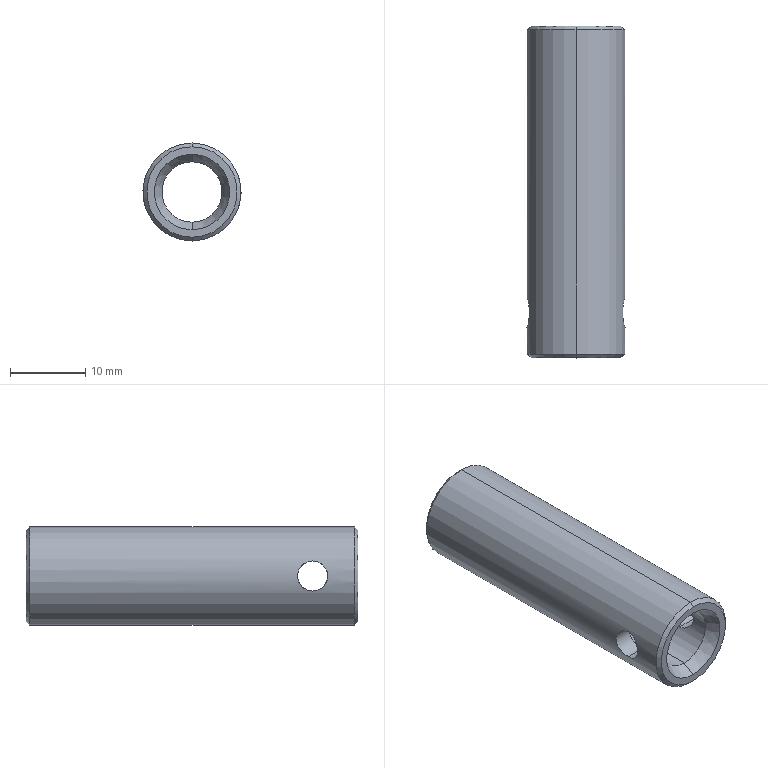Part | SolidWorks | features Chamfer 2, 3DProfileFeature 1, Extrusion 1, HoleWzd 1 | 1 solid | 18 faces | box 13 x 44 x 13 mm | volume 3507 mm3 | cone 8 | cylinder 8 | plane 2 | commonest cylinder face diameters 4 x4 8 x2 13 x2
STEP:
#1=CARTESIAN_POINT('',(0.,42.268,-4.));
#2=VERTEX_POINT('',#1);
#3=CARTESIAN_POINT('',(0.,42.268,4.));
#4=VERTEX_POINT('',#3);
#5=CARTESIAN_POINT('',(0.,42.268,0.));
#6=DIRECTION('',(0.,1.,0.));
#7=DIRECTION('',(0.,0.,1.));
#8=AXIS2_PLACEMENT_3D('',#5,#6,#7);
#9=CIRCLE('',#8,4.);
#10=EDGE_CURVE('',#2,#4,#9,.T.);
#11=ORIENTED_EDGE('',*,*,#10,.F.);
#12=CARTESIAN_POINT('',(0.,44.,-5.));
#13=VERTEX_POINT('',#12);
#14=CARTESIAN_POINT('',(0.,42.268,-4.));
#15=DIRECTION('',(0.,0.866,-0.5));
#16=VECTOR('',#15,1000.);
#17=LINE('',#14,#16);
#18=EDGE_CURVE('',#2,#13,#17,.T.);
#19=ORIENTED_EDGE('',*,*,#18,.T.);
#20=CARTESIAN_POINT('',(0.,44.,5.));
#21=VERTEX_POINT('',#20);
#22=CARTESIAN_POINT('',(0.,44.,0.));
#23=DIRECTION('',(0.,-1.,0.));
#24=DIRECTION('',(0.,0.,1.));
#25=AXIS2_PLACEMENT_3D('',#22,#23,#24);
#26=CIRCLE('',#25,5.);
#27=EDGE_CURVE('',#21,#13,#26,.T.);
#28=ORIENTED_EDGE('',*,*,#27,.F.);
#29=CARTESIAN_POINT('',(0.,42.268,4.));
#30=DIRECTION('',(0.,0.866,0.5));
#31=VECTOR('',#30,1000.);
#32=LINE('',#29,#31);
#33=EDGE_CURVE('',#4,#21,#32,.T.);
#34=ORIENTED_EDGE('',*,*,#33,.F.);
#35=EDGE_LOOP('',(#11,#19,#28,#34));
#36=FACE_OUTER_BOUND('',#35,.T.);
#37=CARTESIAN_POINT('',(0.,42.268,0.));
#38=DIRECTION('',(0.,1.,0.));
#39=DIRECTION('',(0.,0.,1.));
#40=AXIS2_PLACEMENT_3D('',#37,#38,#39);
#41=CONICAL_SURFACE('',#40,4.,0.5236);
#42=ADVANCED_FACE('',(#36),#41,.F.);
#43=CARTESIAN_POINT('',(0.,1.732,4.));
#44=VERTEX_POINT('',#43);
#45=CARTESIAN_POINT('',(0.,1.732,-4.));
#46=VERTEX_POINT('',#45);
#47=CARTESIAN_POINT('',(0.,1.732,0.));
#48=DIRECTION('',(0.,-1.,0.));
#49=DIRECTION('',(0.,0.,1.));
#50=AXIS2_PLACEMENT_3D('',#47,#48,#49);
#51=CIRCLE('',#50,4.);
#52=EDGE_CURVE('',#44,#46,#51,.T.);
#53=ORIENTED_EDGE('',*,*,#52,.F.);
#54=CARTESIAN_POINT('',(0.,0.,5.));
#55=VERTEX_POINT('',#54);
#56=CARTESIAN_POINT('',(0.,0.,5.));
#57=DIRECTION('',(0.,-0.866,0.5));
#58=VECTOR('',#57,1000.);
#59=LINE('',#56,#58);
#60=EDGE_CURVE('',#44,#55,#59,.T.);
#61=ORIENTED_EDGE('',*,*,#60,.T.);
#62=CARTESIAN_POINT('',(0.,0.,-5.));
#63=VERTEX_POINT('',#62);
#64=CARTESIAN_POINT('',(0.,0.,0.));
#65=DIRECTION('',(0.,1.,0.));
#66=DIRECTION('',(0.,0.,1.));
#67=AXIS2_PLACEMENT_3D('',#64,#65,#66);
#68=CIRCLE('',#67,5.);
#69=EDGE_CURVE('',#63,#55,#68,.T.);
#70=ORIENTED_EDGE('',*,*,#69,.F.);
#71=CARTESIAN_POINT('',(0.,0.,-5.));
#72=DIRECTION('',(0.,-0.866,-0.5));
#73=VECTOR('',#72,1000.);
#74=LINE('',#71,#73);
#75=EDGE_CURVE('',#46,#63,#74,.T.);
#76=ORIENTED_EDGE('',*,*,#75,.F.);
#77=EDGE_LOOP('',(#53,#61,#70,#76));
#78=FACE_OUTER_BOUND('',#77,.T.);
#79=CARTESIAN_POINT('',(0.,0.,0.));
#80=DIRECTION('',(0.,-1.,0.));
#81=DIRECTION('',(0.,0.,-1.));
#82=AXIS2_PLACEMENT_3D('',#79,#80,#81);
#83=CONICAL_SURFACE('',#82,5.,0.5236);
#84=ADVANCED_FACE('',(#78),#83,.F.);
#85=CARTESIAN_POINT('',(0.,44.,6.));
#86=VERTEX_POINT('',#85);
#87=CARTESIAN_POINT('',(0.,44.,-6.));
#88=VERTEX_POINT('',#87);
#89=CARTESIAN_POINT('',(0.,44.,0.));
#90=DIRECTION('',(0.,1.,0.));
#91=DIRECTION('',(0.,0.,1.));
#92=AXIS2_PLACEMENT_3D('',#89,#90,#91);
#93=CIRCLE('',#92,6.);
#94=EDGE_CURVE('',#86,#88,#93,.T.);
#95=ORIENTED_EDGE('',*,*,#94,.F.);
#96=CARTESIAN_POINT('',(0.,43.5,6.5));
#97=VERTEX_POINT('',#96);
#98=CARTESIAN_POINT('',(0.,44.,6.));
#99=DIRECTION('',(0.,-0.7071,0.7071));
#100=VECTOR('',#99,1000.);
#101=LINE('',#98,#100);
#102=EDGE_CURVE('',#86,#97,#101,.T.);
#103=ORIENTED_EDGE('',*,*,#102,.T.);
#104=CARTESIAN_POINT('',(0.,43.5,-6.5));
#105=VERTEX_POINT('',#104);
#106=CARTESIAN_POINT('',(0.,43.5,0.));
#107=DIRECTION('',(0.,-1.,0.));
#108=DIRECTION('',(0.,0.,1.));
#109=AXIS2_PLACEMENT_3D('',#106,#107,#108);
#110=CIRCLE('',#109,6.5);
#111=EDGE_CURVE('',#105,#97,#110,.T.);
#112=ORIENTED_EDGE('',*,*,#111,.F.);
#113=CARTESIAN_POINT('',(0.,44.,-6.));
#114=DIRECTION('',(0.,-0.7071,-0.7071));
#115=VECTOR('',#114,1000.);
#116=LINE('',#113,#115);
#117=EDGE_CURVE('',#88,#105,#116,.T.);
#118=ORIENTED_EDGE('',*,*,#117,.F.);
#119=EDGE_LOOP('',(#95,#103,#112,#118));
#120=FACE_OUTER_BOUND('',#119,.T.);
#121=CARTESIAN_POINT('',(0.,44.,0.));
#122=DIRECTION('',(0.,-1.,0.));
#123=DIRECTION('',(0.,0.,-1.));
#124=AXIS2_PLACEMENT_3D('',#121,#122,#123);
#125=CONICAL_SURFACE('',#124,6.,0.7854);
#126=ADVANCED_FACE('',(#120),#125,.T.);
#127=CARTESIAN_POINT('',(0.,0.,-6.));
#128=VERTEX_POINT('',#127);
#129=CARTESIAN_POINT('',(0.,0.,6.));
#130=VERTEX_POINT('',#129);
#131=CARTESIAN_POINT('',(0.,0.,0.));
#132=DIRECTION('',(0.,-1.,0.));
#133=DIRECTION('',(0.,0.,1.));
#134=AXIS2_PLACEMENT_3D('',#131,#132,#133);
#135=CIRCLE('',#134,6.);
#136=EDGE_CURVE('',#128,#130,#135,.T.);
#137=ORIENTED_EDGE('',*,*,#136,.F.);
#138=CARTESIAN_POINT('',(0.,0.5,-6.5));
#139=VERTEX_POINT('',#138);
#140=CARTESIAN_POINT('',(0.,0.5,-6.5));
#141=DIRECTION('',(0.,0.7071,-0.7071));
#142=VECTOR('',#141,1000.);
#143=LINE('',#140,#142);
#144=EDGE_CURVE('',#128,#139,#143,.T.);
#145=ORIENTED_EDGE('',*,*,#144,.T.);
#146=CARTESIAN_POINT('',(0.,0.5,6.5));
#147=VERTEX_POINT('',#146);
#148=CARTESIAN_POINT('',(0.,0.5,0.));
#149=DIRECTION('',(0.,1.,0.));
#150=DIRECTION('',(0.,0.,1.));
#151=AXIS2_PLACEMENT_3D('',#148,#149,#150);
#152=CIRCLE('',#151,6.5);
#153=EDGE_CURVE('',#147,#139,#152,.T.);
#154=ORIENTED_EDGE('',*,*,#153,.F.);
#155=CARTESIAN_POINT('',(0.,0.5,6.5));
#156=DIRECTION('',(0.,0.7071,0.7071));
#157=VECTOR('',#156,1000.);
#158=LINE('',#155,#157);
#159=EDGE_CURVE('',#130,#147,#158,.T.);
#160=ORIENTED_EDGE('',*,*,#159,.F.);
#161=EDGE_LOOP('',(#137,#145,#154,#160));
#162=FACE_OUTER_BOUND('',#161,.T.);
#163=CARTESIAN_POINT('',(0.,0.5,0.));
#164=DIRECTION('',(0.,1.,0.));
#165=DIRECTION('',(0.,0.,1.));
#166=AXIS2_PLACEMENT_3D('',#163,#164,#165);
#167=CONICAL_SURFACE('',#166,6.5,0.7854);
#168=ADVANCED_FACE('',(#162),#167,.T.);
#169=CARTESIAN_POINT('',(-6.185,6.,2.));
#170=VERTEX_POINT('',#169);
#171=CARTESIAN_POINT('',(-6.185,6.,-2.));
#172=VERTEX_POINT('',#171);
#173=CARTESIAN_POINT('',(-6.185,6.,2.));
#174=CARTESIAN_POINT('',(-6.185,5.868,2.));
#175=CARTESIAN_POINT('',(-6.189,5.738,1.987));
#176=CARTESIAN_POINT('',(-6.205,5.48,1.936));
#177=CARTESIAN_POINT('',(-6.217,5.352,1.897));
#178=CARTESIAN_POINT('',(-6.262,4.991,1.746));
#179=CARTESIAN_POINT('',(-6.303,4.769,1.598));
#180=CARTESIAN_POINT('',(-6.365,4.494,1.323));
#181=CARTESIAN_POINT('',(-6.385,4.41,1.221));
#182=CARTESIAN_POINT('',(-6.423,4.265,1.004));
#183=CARTESIAN_POINT('',(-6.44,4.204,0.8894));
#184=CARTESIAN_POINT('',(-6.469,4.103,0.6479));
#185=CARTESIAN_POINT('',(-6.48,4.064,0.5202));
#186=CARTESIAN_POINT('',(-6.496,4.013,0.2629));
#187=CARTESIAN_POINT('',(-6.5,4.,0.1321));
#188=CARTESIAN_POINT('',(-6.5,4.,-0.1339));
#189=CARTESIAN_POINT('',(-6.496,4.013,-0.2646));
#190=CARTESIAN_POINT('',(-6.48,4.065,-0.5213));
#191=CARTESIAN_POINT('',(-6.469,4.104,-0.6488));
#192=CARTESIAN_POINT('',(-6.44,4.204,-0.8906));
#193=CARTESIAN_POINT('',(-6.423,4.266,-1.005));
#194=CARTESIAN_POINT('',(-6.385,4.411,-1.222));
#195=CARTESIAN_POINT('',(-6.364,4.495,-1.324));
#196=CARTESIAN_POINT('',(-6.303,4.77,-1.599));
#197=CARTESIAN_POINT('',(-6.262,4.992,-1.747));
#198=CARTESIAN_POINT('',(-6.217,5.353,-1.897));
#199=CARTESIAN_POINT('',(-6.205,5.48,-1.936));
#200=CARTESIAN_POINT('',(-6.189,5.738,-1.987));
#201=CARTESIAN_POINT('',(-6.185,5.869,-2.));
#202=CARTESIAN_POINT('',(-6.185,6.,-2.));
#203=B_SPLINE_CURVE_WITH_KNOTS('',3,(#173,#174,#175,#176,#177,#178,#179,#180,#181,#182,#183,#184,#185,#186,#187,#188,#189,#190,#191,#192,#193,#194,#195,#196,#197,#198,#199,#200,#201,#202),.UNSPECIFIED.,.F.,.F.,(4,2,2,2,2,2,2,2,2,2,2,2,2,2,4),(0.009436,0.009829,0.01022,0.01101,0.0114,0.0118,0.01219,0.01258,0.01298,0.01337,0.01376,0.01415,0.01494,0.01533,0.01573),.UNSPECIFIED.);
#204=EDGE_CURVE('',#170,#172,#203,.T.);
#205=ORIENTED_EDGE('',*,*,#204,.F.);
#206=CARTESIAN_POINT('',(-3.464,6.,2.));
#207=VERTEX_POINT('',#206);
#208=CARTESIAN_POINT('',(6.5,6.,2.));
#209=DIRECTION('',(1.,0.,0.));
#210=VECTOR('',#209,1000.);
#211=LINE('',#208,#210);
#212=EDGE_CURVE('',#170,#207,#211,.T.);
#213=ORIENTED_EDGE('',*,*,#212,.T.);
#214=CARTESIAN_POINT('',(-3.464,6.,-2.));
#215=VERTEX_POINT('',#214);
#216=CARTESIAN_POINT('',(-3.464,6.,2.));
#217=CARTESIAN_POINT('',(-3.464,5.868,2.));
#218=CARTESIAN_POINT('',(-3.472,5.733,1.986));
#219=CARTESIAN_POINT('',(-3.501,5.474,1.934));
#220=CARTESIAN_POINT('',(-3.523,5.348,1.895));
#221=CARTESIAN_POINT('',(-3.576,5.105,1.794));
#222=CARTESIAN_POINT('',(-3.606,4.991,1.732));
#223=CARTESIAN_POINT('',(-3.672,4.778,1.588));
#224=CARTESIAN_POINT('',(-3.707,4.677,1.505));
#225=CARTESIAN_POINT('',(-3.776,4.495,1.324));
#226=CARTESIAN_POINT('',(-3.81,4.413,1.225));
#227=CARTESIAN_POINT('',(-3.872,4.269,1.01));
#228=CARTESIAN_POINT('',(-3.901,4.206,0.8936));
#229=CARTESIAN_POINT('',(-3.972,4.055,0.5337));
#230=CARTESIAN_POINT('',(-4.,4.,0.2665));
#231=CARTESIAN_POINT('',(-4.,4.,-0.1307));
#232=CARTESIAN_POINT('',(-3.993,4.013,-0.265));
#233=CARTESIAN_POINT('',(-3.967,4.066,-0.5254));
#234=CARTESIAN_POINT('',(-3.949,4.104,-0.651));
#235=CARTESIAN_POINT('',(-3.877,4.257,-1.015));
#236=CARTESIAN_POINT('',(-3.81,4.404,-1.233));
#237=CARTESIAN_POINT('',(-3.707,4.678,-1.507));
#238=CARTESIAN_POINT('',(-3.672,4.777,-1.588));
#239=CARTESIAN_POINT('',(-3.607,4.991,-1.732));
#240=CARTESIAN_POINT('',(-3.575,5.107,-1.794));
#241=CARTESIAN_POINT('',(-3.523,5.347,-1.895));
#242=CARTESIAN_POINT('',(-3.502,5.471,-1.933));
#243=CARTESIAN_POINT('',(-3.472,5.731,-1.986));
#244=CARTESIAN_POINT('',(-3.464,5.866,-2.));
#245=CARTESIAN_POINT('',(-3.464,6.,-2.));
#246=B_SPLINE_CURVE_WITH_KNOTS('',3,(#216,#217,#218,#219,#220,#221,#222,#223,#224,#225,#226,#227,#228,#229,#230,#231,#232,#233,#234,#235,#236,#237,#238,#239,#240,#241,#242,#243,#244,#245),.UNSPECIFIED.,.F.,.F.,(4,2,2,2,2,2,2,2,2,2,2,2,2,2,4),(0.006361,0.006758,0.007155,0.007552,0.007949,0.008346,0.008742,0.009536,0.009933,0.01033,0.01112,0.01152,0.01192,0.01231,0.01271),.UNSPECIFIED.);
#247=EDGE_CURVE('',#207,#215,#246,.T.);
#248=ORIENTED_EDGE('',*,*,#247,.T.);
#249=CARTESIAN_POINT('',(6.5,6.,-2.));
#250=DIRECTION('',(1.,0.,0.));
#251=VECTOR('',#250,1000.);
#252=LINE('',#249,#251);
#253=EDGE_CURVE('',#172,#215,#252,.T.);
#254=ORIENTED_EDGE('',*,*,#253,.F.);
#255=EDGE_LOOP('',(#205,#213,#248,#254));
#256=FACE_OUTER_BOUND('',#255,.T.);
#257=CARTESIAN_POINT('',(6.5,6.,0.));
#258=DIRECTION('',(1.,0.,0.));
#259=DIRECTION('',(0.,0.,-1.));
#260=AXIS2_PLACEMENT_3D('',#257,#258,#259);
#261=CYLINDRICAL_SURFACE('',#260,2.);
#262=ADVANCED_FACE('',(#256),#261,.F.);
#263=CARTESIAN_POINT('',(3.464,6.,-2.));
#264=VERTEX_POINT('',#263);
#265=CARTESIAN_POINT('',(3.464,6.,2.));
#266=VERTEX_POINT('',#265);
#267=CARTESIAN_POINT('',(3.464,6.,-2.));
#268=CARTESIAN_POINT('',(3.464,5.865,-2.));
#269=CARTESIAN_POINT('',(3.472,5.733,-1.987));
#270=CARTESIAN_POINT('',(3.501,5.475,-1.934));
#271=CARTESIAN_POINT('',(3.523,5.347,-1.895));
#272=CARTESIAN_POINT('',(3.602,4.986,-1.743));
#273=CARTESIAN_POINT('',(3.673,4.768,-1.596));
#274=CARTESIAN_POINT('',(3.81,4.405,-1.233));
#275=CARTESIAN_POINT('',(3.877,4.257,-1.014));
#276=CARTESIAN_POINT('',(3.948,4.105,-0.6539));
#277=CARTESIAN_POINT('',(3.967,4.066,-0.5256));
#278=CARTESIAN_POINT('',(3.993,4.013,-0.2661));
#279=CARTESIAN_POINT('',(4.,4.,-0.1346));
#280=CARTESIAN_POINT('',(4.,4.,0.132));
#281=CARTESIAN_POINT('',(3.993,4.013,0.2666));
#282=CARTESIAN_POINT('',(3.967,4.066,0.5257));
#283=CARTESIAN_POINT('',(3.948,4.105,0.653));
#284=CARTESIAN_POINT('',(3.9,4.207,0.8959));
#285=CARTESIAN_POINT('',(3.872,4.269,1.01));
#286=CARTESIAN_POINT('',(3.809,4.414,1.225));
#287=CARTESIAN_POINT('',(3.775,4.497,1.326));
#288=CARTESIAN_POINT('',(3.672,4.77,1.598));
#289=CARTESIAN_POINT('',(3.601,4.989,1.745));
#290=CARTESIAN_POINT('',(3.523,5.348,1.895));
#291=CARTESIAN_POINT('',(3.501,5.475,1.934));
#292=CARTESIAN_POINT('',(3.472,5.736,1.987));
#293=CARTESIAN_POINT('',(3.464,5.867,2.));
#294=CARTESIAN_POINT('',(3.464,6.,2.));
#295=B_SPLINE_CURVE_WITH_KNOTS('',3,(#267,#268,#269,#270,#271,#272,#273,#274,#275,#276,#277,#278,#279,#280,#281,#282,#283,#284,#285,#286,#287,#288,#289,#290,#291,#292,#293,#294),.UNSPECIFIED.,.F.,.F.,(4,2,2,2,2,2,2,2,2,2,2,2,2,4),(0.,0.0003976,0.0007951,0.00159,0.002385,0.002783,0.003181,0.003578,0.003976,0.004373,0.004771,0.005566,0.005964,0.006361),.UNSPECIFIED.);
#296=EDGE_CURVE('',#264,#266,#295,.T.);
#297=ORIENTED_EDGE('',*,*,#296,.T.);
#298=CARTESIAN_POINT('',(6.185,6.,2.));
#299=VERTEX_POINT('',#298);
#300=CARTESIAN_POINT('',(6.5,6.,2.));
#301=DIRECTION('',(1.,0.,0.));
#302=VECTOR('',#301,1000.);
#303=LINE('',#300,#302);
#304=EDGE_CURVE('',#266,#299,#303,.T.);
#305=ORIENTED_EDGE('',*,*,#304,.T.);
#306=CARTESIAN_POINT('',(6.185,6.,-2.));
#307=VERTEX_POINT('',#306);
#308=CARTESIAN_POINT('',(6.185,6.,-2.));
#309=CARTESIAN_POINT('',(6.185,5.867,-2.));
#310=CARTESIAN_POINT('',(6.189,5.736,-1.987));
#311=CARTESIAN_POINT('',(6.205,5.48,-1.936));
#312=CARTESIAN_POINT('',(6.217,5.352,-1.897));
#313=CARTESIAN_POINT('',(6.247,5.11,-1.796));
#314=CARTESIAN_POINT('',(6.265,4.996,-1.735));
#315=CARTESIAN_POINT('',(6.303,4.779,-1.589));
#316=CARTESIAN_POINT('',(6.324,4.677,-1.506));
#317=CARTESIAN_POINT('',(6.385,4.402,-1.231));
#318=CARTESIAN_POINT('',(6.426,4.254,-1.009));
#319=CARTESIAN_POINT('',(6.469,4.103,-0.6481));
#320=CARTESIAN_POINT('',(6.48,4.065,-0.5212));
#321=CARTESIAN_POINT('',(6.496,4.013,-0.2626));
#322=CARTESIAN_POINT('',(6.5,4.,-0.1323));
#323=CARTESIAN_POINT('',(6.5,4.,0.1305));
#324=CARTESIAN_POINT('',(6.496,4.013,0.2639));
#325=CARTESIAN_POINT('',(6.48,4.065,0.5212));
#326=CARTESIAN_POINT('',(6.469,4.103,0.6463));
#327=CARTESIAN_POINT('',(6.426,4.254,1.011));
#328=CARTESIAN_POINT('',(6.385,4.402,1.231));
#329=CARTESIAN_POINT('',(6.324,4.679,1.507));
#330=CARTESIAN_POINT('',(6.303,4.779,1.589));
#331=CARTESIAN_POINT('',(6.265,4.995,1.734));
#332=CARTESIAN_POINT('',(6.247,5.112,1.797));
#333=CARTESIAN_POINT('',(6.217,5.353,1.897));
#334=CARTESIAN_POINT('',(6.205,5.478,1.935));
#335=CARTESIAN_POINT('',(6.189,5.736,1.987));
#336=CARTESIAN_POINT('',(6.185,5.869,2.));
#337=CARTESIAN_POINT('',(6.185,6.,2.));
#338=B_SPLINE_CURVE_WITH_KNOTS('',3,(#308,#309,#310,#311,#312,#313,#314,#315,#316,#317,#318,#319,#320,#321,#322,#323,#324,#325,#326,#327,#328,#329,#330,#331,#332,#333,#334,#335,#336,#337),.UNSPECIFIED.,.F.,.F.,(4,2,2,2,2,2,2,2,2,2,2,2,2,2,4),(0.,0.0003932,0.0007864,0.00118,0.001573,0.002359,0.002752,0.003146,0.003539,0.003932,0.004718,0.005112,0.005505,0.005898,0.006291),.UNSPECIFIED.);
#339=EDGE_CURVE('',#307,#299,#338,.T.);
#340=ORIENTED_EDGE('',*,*,#339,.F.);
#341=CARTESIAN_POINT('',(6.5,6.,-2.));
#342=DIRECTION('',(1.,0.,0.));
#343=VECTOR('',#342,1000.);
#344=LINE('',#341,#343);
#345=EDGE_CURVE('',#264,#307,#344,.T.);
#346=ORIENTED_EDGE('',*,*,#345,.F.);
#347=EDGE_LOOP('',(#297,#305,#340,#346));
#348=FACE_OUTER_BOUND('',#347,.T.);
#349=CARTESIAN_POINT('',(6.5,6.,0.));
#350=DIRECTION('',(1.,0.,0.));
#351=DIRECTION('',(0.,0.,-1.));
#352=AXIS2_PLACEMENT_3D('',#349,#350,#351);
#353=CYLINDRICAL_SURFACE('',#352,2.);
#354=ADVANCED_FACE('',(#348),#353,.F.);
#355=CARTESIAN_POINT('',(-3.464,6.,-2.));
#356=CARTESIAN_POINT('',(-3.464,6.135,-2.));
#357=CARTESIAN_POINT('',(-3.472,6.267,-1.987));
#358=CARTESIAN_POINT('',(-3.501,6.525,-1.934));
#359=CARTESIAN_POINT('',(-3.523,6.653,-1.895));
#360=CARTESIAN_POINT('',(-3.602,7.014,-1.743));
#361=CARTESIAN_POINT('',(-3.673,7.232,-1.596));
#362=CARTESIAN_POINT('',(-3.81,7.595,-1.233));
#363=CARTESIAN_POINT('',(-3.877,7.743,-1.014));
#364=CARTESIAN_POINT('',(-3.948,7.895,-0.6539));
#365=CARTESIAN_POINT('',(-3.967,7.934,-0.5256));
#366=CARTESIAN_POINT('',(-3.993,7.987,-0.2661));
#367=CARTESIAN_POINT('',(-4.,8.,-0.1346));
#368=CARTESIAN_POINT('',(-4.,8.,0.132));
#369=CARTESIAN_POINT('',(-3.993,7.987,0.2666));
#370=CARTESIAN_POINT('',(-3.967,7.934,0.5257));
#371=CARTESIAN_POINT('',(-3.948,7.895,0.653));
#372=CARTESIAN_POINT('',(-3.9,7.793,0.8959));
#373=CARTESIAN_POINT('',(-3.872,7.731,1.01));
#374=CARTESIAN_POINT('',(-3.809,7.586,1.225));
#375=CARTESIAN_POINT('',(-3.775,7.503,1.326));
#376=CARTESIAN_POINT('',(-3.672,7.23,1.598));
#377=CARTESIAN_POINT('',(-3.601,7.011,1.745));
#378=CARTESIAN_POINT('',(-3.523,6.652,1.895));
#379=CARTESIAN_POINT('',(-3.501,6.525,1.934));
#380=CARTESIAN_POINT('',(-3.472,6.264,1.987));
#381=CARTESIAN_POINT('',(-3.464,6.133,2.));
#382=CARTESIAN_POINT('',(-3.464,6.,2.));
#383=B_SPLINE_CURVE_WITH_KNOTS('',3,(#355,#356,#357,#358,#359,#360,#361,#362,#363,#364,#365,#366,#367,#368,#369,#370,#371,#372,#373,#374,#375,#376,#377,#378,#379,#380,#381,#382),.UNSPECIFIED.,.F.,.F.,(4,2,2,2,2,2,2,2,2,2,2,2,2,4),(0.,0.0003976,0.0007951,0.00159,0.002385,0.002783,0.003181,0.003578,0.003976,0.004373,0.004771,0.005566,0.005964,0.006361),.UNSPECIFIED.);
#384=EDGE_CURVE('',#215,#207,#383,.T.);
#385=ORIENTED_EDGE('',*,*,#384,.F.);
#386=ORIENTED_EDGE('',*,*,#247,.F.);
#387=EDGE_LOOP('',(#385,#386));
#388=FACE_BOUND('',#387,.T.);
#389=ORIENTED_EDGE('',*,*,#10,.T.);
#390=CARTESIAN_POINT('',(0.,44.,4.));
#391=DIRECTION('',(0.,-1.,0.));
#392=VECTOR('',#391,1000.);
#393=LINE('',#390,#392);
#394=EDGE_CURVE('',#4,#44,#393,.T.);
#395=ORIENTED_EDGE('',*,*,#394,.T.);
#396=ORIENTED_EDGE('',*,*,#52,.T.);
#397=CARTESIAN_POINT('',(0.,44.,-4.));
#398=DIRECTION('',(0.,-1.,0.));
#399=VECTOR('',#398,1000.);
#400=LINE('',#397,#399);
#401=EDGE_CURVE('',#2,#46,#400,.T.);
#402=ORIENTED_EDGE('',*,*,#401,.F.);
#403=EDGE_LOOP('',(#389,#395,#396,#402));
#404=FACE_OUTER_BOUND('',#403,.T.);
#405=CARTESIAN_POINT('',(0.,44.,0.));
#406=DIRECTION('',(0.,-1.,0.));
#407=DIRECTION('',(0.,0.,-1.));
#408=AXIS2_PLACEMENT_3D('',#405,#406,#407);
#409=CYLINDRICAL_SURFACE('',#408,4.);
#410=ADVANCED_FACE('',(#388,#404),#409,.F.);
#411=ORIENTED_EDGE('',*,*,#339,.T.);
#412=CARTESIAN_POINT('',(6.185,6.,2.));
#413=CARTESIAN_POINT('',(6.185,6.262,2.));
#414=CARTESIAN_POINT('',(6.202,6.527,1.947));
#415=CARTESIAN_POINT('',(6.247,6.888,1.797));
#416=CARTESIAN_POINT('',(6.265,7.005,1.734));
#417=CARTESIAN_POINT('',(6.303,7.221,1.589));
#418=CARTESIAN_POINT('',(6.324,7.322,1.507));
#419=CARTESIAN_POINT('',(6.385,7.599,1.23));
#420=CARTESIAN_POINT('',(6.425,7.745,1.012));
#421=CARTESIAN_POINT('',(6.469,7.897,0.6464));
#422=CARTESIAN_POINT('',(6.48,7.935,0.5213));
#423=CARTESIAN_POINT('',(6.496,7.987,0.2649));
#424=CARTESIAN_POINT('',(6.5,8.,0.1318));
#425=CARTESIAN_POINT('',(6.5,8.,-0.1318));
#426=CARTESIAN_POINT('',(6.496,7.987,-0.2621));
#427=CARTESIAN_POINT('',(6.48,7.936,-0.52));
#428=CARTESIAN_POINT('',(6.469,7.897,-0.6476));
#429=CARTESIAN_POINT('',(6.426,7.746,-1.009));
#430=CARTESIAN_POINT('',(6.385,7.598,-1.231));
#431=CARTESIAN_POINT('',(6.324,7.323,-1.506));
#432=CARTESIAN_POINT('',(6.303,7.221,-1.59));
#433=CARTESIAN_POINT('',(6.265,7.004,-1.735));
#434=CARTESIAN_POINT('',(6.247,6.89,-1.796));
#435=CARTESIAN_POINT('',(6.217,6.649,-1.896));
#436=CARTESIAN_POINT('',(6.205,6.521,-1.935));
#437=CARTESIAN_POINT('',(6.189,6.264,-1.987));
#438=CARTESIAN_POINT('',(6.185,6.133,-2.));
#439=CARTESIAN_POINT('',(6.185,6.,-2.));
#440=B_SPLINE_CURVE_WITH_KNOTS('',3,(#412,#413,#414,#415,#416,#417,#418,#419,#420,#421,#422,#423,#424,#425,#426,#427,#428,#429,#430,#431,#432,#433,#434,#435,#436,#437,#438,#439),.UNSPECIFIED.,.F.,.F.,(4,2,2,2,2,2,2,2,2,2,2,2,2,4),(0.006291,0.007077,0.00747,0.007864,0.00865,0.009043,0.009436,0.009829,0.01022,0.01101,0.0114,0.01179,0.01219,0.01258),.UNSPECIFIED.);
#441=EDGE_CURVE('',#299,#307,#440,.T.);
#442=ORIENTED_EDGE('',*,*,#441,.T.);
#443=EDGE_LOOP('',(#411,#442));
#444=FACE_BOUND('',#443,.T.);
#445=ORIENTED_EDGE('',*,*,#111,.T.);
#446=CARTESIAN_POINT('',(0.,44.,6.5));
#447=DIRECTION('',(0.,-1.,0.));
#448=VECTOR('',#447,1000.);
#449=LINE('',#446,#448);
#450=EDGE_CURVE('',#97,#147,#449,.T.);
#451=ORIENTED_EDGE('',*,*,#450,.T.);
#452=ORIENTED_EDGE('',*,*,#153,.T.);
#453=CARTESIAN_POINT('',(0.,44.,-6.5));
#454=DIRECTION('',(0.,-1.,0.));
#455=VECTOR('',#454,1000.);
#456=LINE('',#453,#455);
#457=EDGE_CURVE('',#105,#139,#456,.T.);
#458=ORIENTED_EDGE('',*,*,#457,.F.);
#459=EDGE_LOOP('',(#445,#451,#452,#458));
#460=FACE_OUTER_BOUND('',#459,.T.);
#461=CARTESIAN_POINT('',(0.,44.,0.));
#462=DIRECTION('',(0.,-1.,0.));
#463=DIRECTION('',(0.,0.,-1.));
#464=AXIS2_PLACEMENT_3D('',#461,#462,#463);
#465=CYLINDRICAL_SURFACE('',#464,6.5);
#466=ADVANCED_FACE('',(#444,#460),#465,.T.);
#467=ORIENTED_EDGE('',*,*,#27,.T.);
#468=CARTESIAN_POINT('',(0.,44.,0.));
#469=DIRECTION('',(0.,-1.,0.));
#470=DIRECTION('',(0.,0.,1.));
#471=AXIS2_PLACEMENT_3D('',#468,#469,#470);
#472=CIRCLE('',#471,5.);
#473=EDGE_CURVE('',#13,#21,#472,.T.);
#474=ORIENTED_EDGE('',*,*,#473,.T.);
#475=EDGE_LOOP('',(#467,#474));
#476=FACE_BOUND('',#475,.T.);
#477=CARTESIAN_POINT('',(0.,44.,0.));
#478=DIRECTION('',(0.,1.,0.));
#479=DIRECTION('',(0.,0.,1.));
#480=AXIS2_PLACEMENT_3D('',#477,#478,#479);
#481=CIRCLE('',#480,6.);
#482=EDGE_CURVE('',#88,#86,#481,.T.);
#483=ORIENTED_EDGE('',*,*,#482,.T.);
#484=ORIENTED_EDGE('',*,*,#94,.T.);
#485=EDGE_LOOP('',(#483,#484));
#486=FACE_OUTER_BOUND('',#485,.T.);
#487=CARTESIAN_POINT('',(0.,44.,0.));
#488=DIRECTION('',(0.,1.,0.));
#489=DIRECTION('',(0.,0.,1.));
#490=AXIS2_PLACEMENT_3D('',#487,#488,#489);
#491=PLANE('',#490);
#492=ADVANCED_FACE('',(#476,#486),#491,.T.);
#493=ORIENTED_EDGE('',*,*,#69,.T.);
#494=CARTESIAN_POINT('',(0.,0.,0.));
#495=DIRECTION('',(0.,1.,0.));
#496=DIRECTION('',(0.,0.,1.));
#497=AXIS2_PLACEMENT_3D('',#494,#495,#496);
#498=CIRCLE('',#497,5.);
#499=EDGE_CURVE('',#55,#63,#498,.T.);
#500=ORIENTED_EDGE('',*,*,#499,.T.);
#501=EDGE_LOOP('',(#493,#500));
#502=FACE_BOUND('',#501,.T.);
#503=CARTESIAN_POINT('',(0.,0.,0.));
#504=DIRECTION('',(0.,-1.,0.));
#505=DIRECTION('',(0.,0.,1.));
#506=AXIS2_PLACEMENT_3D('',#503,#504,#505);
#507=CIRCLE('',#506,6.);
#508=EDGE_CURVE('',#130,#128,#507,.T.);
#509=ORIENTED_EDGE('',*,*,#508,.T.);
#510=ORIENTED_EDGE('',*,*,#136,.T.);
#511=EDGE_LOOP('',(#509,#510));
#512=FACE_OUTER_BOUND('',#511,.T.);
#513=CARTESIAN_POINT('',(0.,0.,0.));
#514=DIRECTION('',(0.,1.,0.));
#515=DIRECTION('',(0.,0.,1.));
#516=AXIS2_PLACEMENT_3D('',#513,#514,#515);
#517=PLANE('',#516);
#518=ADVANCED_FACE('',(#502,#512),#517,.F.);
#519=ORIENTED_EDGE('',*,*,#450,.F.);
#520=CARTESIAN_POINT('',(0.,43.5,0.));
#521=DIRECTION('',(0.,-1.,0.));
#522=DIRECTION('',(0.,0.,1.));
#523=AXIS2_PLACEMENT_3D('',#520,#521,#522);
#524=CIRCLE('',#523,6.5);
#525=EDGE_CURVE('',#97,#105,#524,.T.);
#526=ORIENTED_EDGE('',*,*,#525,.T.);
#527=ORIENTED_EDGE('',*,*,#457,.T.);
#528=CARTESIAN_POINT('',(0.,0.5,0.));
#529=DIRECTION('',(0.,1.,0.));
#530=DIRECTION('',(0.,0.,1.));
#531=AXIS2_PLACEMENT_3D('',#528,#529,#530);
#532=CIRCLE('',#531,6.5);
#533=EDGE_CURVE('',#139,#147,#532,.T.);
#534=ORIENTED_EDGE('',*,*,#533,.T.);
#535=EDGE_LOOP('',(#519,#526,#527,#534));
#536=FACE_OUTER_BOUND('',#535,.T.);
#537=CARTESIAN_POINT('',(-6.185,6.,-2.));
#538=CARTESIAN_POINT('',(-6.185,6.131,-2.));
#539=CARTESIAN_POINT('',(-6.189,6.265,-1.987));
#540=CARTESIAN_POINT('',(-6.205,6.522,-1.935));
#541=CARTESIAN_POINT('',(-6.217,6.647,-1.897));
#542=CARTESIAN_POINT('',(-6.262,7.011,-1.745));
#543=CARTESIAN_POINT('',(-6.303,7.231,-1.598));
#544=CARTESIAN_POINT('',(-6.365,7.507,-1.321));
#545=CARTESIAN_POINT('',(-6.385,7.589,-1.221));
#546=CARTESIAN_POINT('',(-6.423,7.734,-1.005));
#547=CARTESIAN_POINT('',(-6.44,7.797,-0.8878));
#548=CARTESIAN_POINT('',(-6.469,7.897,-0.6468));
#549=CARTESIAN_POINT('',(-6.48,7.935,-0.522));
#550=CARTESIAN_POINT('',(-6.496,7.987,-0.2636));
#551=CARTESIAN_POINT('',(-6.5,8.,-0.1309));
#552=CARTESIAN_POINT('',(-6.5,8.,0.2621));
#553=CARTESIAN_POINT('',(-6.483,7.947,0.5267));
#554=CARTESIAN_POINT('',(-6.44,7.797,0.8884));
#555=CARTESIAN_POINT('',(-6.423,7.734,1.005));
#556=CARTESIAN_POINT('',(-6.385,7.589,1.222));
#557=CARTESIAN_POINT('',(-6.365,7.507,1.322));
#558=CARTESIAN_POINT('',(-6.324,7.322,1.506));
#559=CARTESIAN_POINT('',(-6.303,7.22,1.59));
#560=CARTESIAN_POINT('',(-6.265,7.005,1.734));
#561=CARTESIAN_POINT('',(-6.247,6.89,1.796));
#562=CARTESIAN_POINT('',(-6.217,6.646,1.897));
#563=CARTESIAN_POINT('',(-6.205,6.521,1.935));
#564=CARTESIAN_POINT('',(-6.189,6.265,1.987));
#565=CARTESIAN_POINT('',(-6.185,6.132,2.));
#566=CARTESIAN_POINT('',(-6.185,6.,2.));
#567=B_SPLINE_CURVE_WITH_KNOTS('',3,(#537,#538,#539,#540,#541,#542,#543,#544,#545,#546,#547,#548,#549,#550,#551,#552,#553,#554,#555,#556,#557,#558,#559,#560,#561,#562,#563,#564,#565,#566),.UNSPECIFIED.,.F.,.F.,(4,2,2,2,2,2,2,2,2,2,2,2,2,2,4),(0.003147,0.00354,0.003933,0.004719,0.005112,0.005505,0.005898,0.006291,0.007078,0.007471,0.007864,0.008257,0.00865,0.009043,0.009436),.UNSPECIFIED.);
#568=EDGE_CURVE('',#172,#170,#567,.T.);
#569=ORIENTED_EDGE('',*,*,#568,.T.);
#570=ORIENTED_EDGE('',*,*,#204,.T.);
#571=EDGE_LOOP('',(#569,#570));
#572=FACE_BOUND('',#571,.T.);
#573=CARTESIAN_POINT('',(0.,44.,0.));
#574=DIRECTION('',(0.,-1.,0.));
#575=DIRECTION('',(0.,0.,-1.));
#576=AXIS2_PLACEMENT_3D('',#573,#574,#575);
#577=CYLINDRICAL_SURFACE('',#576,6.5);
#578=ADVANCED_FACE('',(#536,#572),#577,.T.);
#579=ORIENTED_EDGE('',*,*,#394,.F.);
#580=CARTESIAN_POINT('',(0.,42.268,0.));
#581=DIRECTION('',(0.,1.,0.));
#582=DIRECTION('',(0.,0.,1.));
#583=AXIS2_PLACEMENT_3D('',#580,#581,#582);
#584=CIRCLE('',#583,4.);
#585=EDGE_CURVE('',#4,#2,#584,.T.);
#586=ORIENTED_EDGE('',*,*,#585,.T.);
#587=ORIENTED_EDGE('',*,*,#401,.T.);
#588=CARTESIAN_POINT('',(0.,1.732,0.));
#589=DIRECTION('',(0.,-1.,0.));
#590=DIRECTION('',(0.,0.,1.));
#591=AXIS2_PLACEMENT_3D('',#588,#589,#590);
#592=CIRCLE('',#591,4.);
#593=EDGE_CURVE('',#46,#44,#592,.T.);
#594=ORIENTED_EDGE('',*,*,#593,.T.);
#595=EDGE_LOOP('',(#579,#586,#587,#594));
#596=FACE_OUTER_BOUND('',#595,.T.);
#597=ORIENTED_EDGE('',*,*,#296,.F.);
#598=CARTESIAN_POINT('',(3.464,6.,2.));
#599=CARTESIAN_POINT('',(3.464,6.132,2.));
#600=CARTESIAN_POINT('',(3.472,6.267,1.986));
#601=CARTESIAN_POINT('',(3.501,6.526,1.934));
#602=CARTESIAN_POINT('',(3.523,6.652,1.895));
#603=CARTESIAN_POINT('',(3.576,6.895,1.794));
#604=CARTESIAN_POINT('',(3.606,7.009,1.732));
#605=CARTESIAN_POINT('',(3.672,7.222,1.588));
#606=CARTESIAN_POINT('',(3.707,7.323,1.505));
#607=CARTESIAN_POINT('',(3.776,7.505,1.324));
#608=CARTESIAN_POINT('',(3.81,7.587,1.225));
#609=CARTESIAN_POINT('',(3.872,7.731,1.01));
#610=CARTESIAN_POINT('',(3.901,7.794,0.8936));
#611=CARTESIAN_POINT('',(3.972,7.945,0.5337));
#612=CARTESIAN_POINT('',(4.,8.,0.2665));
#613=CARTESIAN_POINT('',(4.,8.,-0.1307));
#614=CARTESIAN_POINT('',(3.993,7.987,-0.265));
#615=CARTESIAN_POINT('',(3.967,7.934,-0.5254));
#616=CARTESIAN_POINT('',(3.949,7.896,-0.651));
#617=CARTESIAN_POINT('',(3.877,7.743,-1.015));
#618=CARTESIAN_POINT('',(3.81,7.596,-1.233));
#619=CARTESIAN_POINT('',(3.707,7.322,-1.507));
#620=CARTESIAN_POINT('',(3.672,7.223,-1.588));
#621=CARTESIAN_POINT('',(3.607,7.009,-1.732));
#622=CARTESIAN_POINT('',(3.575,6.893,-1.794));
#623=CARTESIAN_POINT('',(3.523,6.653,-1.895));
#624=CARTESIAN_POINT('',(3.502,6.529,-1.933));
#625=CARTESIAN_POINT('',(3.472,6.269,-1.986));
#626=CARTESIAN_POINT('',(3.464,6.134,-2.));
#627=CARTESIAN_POINT('',(3.464,6.,-2.));
#628=B_SPLINE_CURVE_WITH_KNOTS('',3,(#598,#599,#600,#601,#602,#603,#604,#605,#606,#607,#608,#609,#610,#611,#612,#613,#614,#615,#616,#617,#618,#619,#620,#621,#622,#623,#624,#625,#626,#627),.UNSPECIFIED.,.F.,.F.,(4,2,2,2,2,2,2,2,2,2,2,2,2,2,4),(0.006361,0.006758,0.007155,0.007552,0.007949,0.008346,0.008742,0.009536,0.009933,0.01033,0.01112,0.01152,0.01192,0.01231,0.01271),.UNSPECIFIED.);
#629=EDGE_CURVE('',#266,#264,#628,.T.);
#630=ORIENTED_EDGE('',*,*,#629,.F.);
#631=EDGE_LOOP('',(#597,#630));
#632=FACE_BOUND('',#631,.T.);
#633=CARTESIAN_POINT('',(0.,44.,0.));
#634=DIRECTION('',(0.,-1.,0.));
#635=DIRECTION('',(0.,0.,-1.));
#636=AXIS2_PLACEMENT_3D('',#633,#634,#635);
#637=CYLINDRICAL_SURFACE('',#636,4.);
#638=ADVANCED_FACE('',(#596,#632),#637,.F.);
#639=ORIENTED_EDGE('',*,*,#304,.F.);
#640=ORIENTED_EDGE('',*,*,#629,.T.);
#641=ORIENTED_EDGE('',*,*,#345,.T.);
#642=ORIENTED_EDGE('',*,*,#441,.F.);
#643=EDGE_LOOP('',(#639,#640,#641,#642));
#644=FACE_OUTER_BOUND('',#643,.T.);
#645=CARTESIAN_POINT('',(6.5,6.,0.));
#646=DIRECTION('',(1.,0.,0.));
#647=DIRECTION('',(0.,0.,-1.));
#648=AXIS2_PLACEMENT_3D('',#645,#646,#647);
#649=CYLINDRICAL_SURFACE('',#648,2.);
#650=ADVANCED_FACE('',(#644),#649,.F.);
#651=ORIENTED_EDGE('',*,*,#212,.F.);
#652=ORIENTED_EDGE('',*,*,#568,.F.);
#653=ORIENTED_EDGE('',*,*,#253,.T.);
#654=ORIENTED_EDGE('',*,*,#384,.T.);
#655=EDGE_LOOP('',(#651,#652,#653,#654));
#656=FACE_OUTER_BOUND('',#655,.T.);
#657=CARTESIAN_POINT('',(6.5,6.,0.));
#658=DIRECTION('',(1.,0.,0.));
#659=DIRECTION('',(0.,0.,-1.));
#660=AXIS2_PLACEMENT_3D('',#657,#658,#659);
#661=CYLINDRICAL_SURFACE('',#660,2.);
#662=ADVANCED_FACE('',(#656),#661,.F.);
#663=ORIENTED_EDGE('',*,*,#144,.F.);
#664=ORIENTED_EDGE('',*,*,#508,.F.);
#665=ORIENTED_EDGE('',*,*,#159,.T.);
#666=ORIENTED_EDGE('',*,*,#533,.F.);
#667=EDGE_LOOP('',(#663,#664,#665,#666));
#668=FACE_OUTER_BOUND('',#667,.T.);
#669=CARTESIAN_POINT('',(0.,0.5,0.));
#670=DIRECTION('',(0.,1.,0.));
#671=DIRECTION('',(0.,0.,1.));
#672=AXIS2_PLACEMENT_3D('',#669,#670,#671);
#673=CONICAL_SURFACE('',#672,6.5,0.7854);
#674=ADVANCED_FACE('',(#668),#673,.T.);
#675=ORIENTED_EDGE('',*,*,#102,.F.);
#676=ORIENTED_EDGE('',*,*,#482,.F.);
#677=ORIENTED_EDGE('',*,*,#117,.T.);
#678=ORIENTED_EDGE('',*,*,#525,.F.);
#679=EDGE_LOOP('',(#675,#676,#677,#678));
#680=FACE_OUTER_BOUND('',#679,.T.);
#681=CARTESIAN_POINT('',(0.,44.,0.));
#682=DIRECTION('',(0.,-1.,0.));
#683=DIRECTION('',(0.,0.,-1.));
#684=AXIS2_PLACEMENT_3D('',#681,#682,#683);
#685=CONICAL_SURFACE('',#684,6.,0.7854);
#686=ADVANCED_FACE('',(#680),#685,.T.);
#687=ORIENTED_EDGE('',*,*,#60,.F.);
#688=ORIENTED_EDGE('',*,*,#593,.F.);
#689=ORIENTED_EDGE('',*,*,#75,.T.);
#690=ORIENTED_EDGE('',*,*,#499,.F.);
#691=EDGE_LOOP('',(#687,#688,#689,#690));
#692=FACE_OUTER_BOUND('',#691,.T.);
#693=CARTESIAN_POINT('',(0.,0.,0.));
#694=DIRECTION('',(0.,-1.,0.));
#695=DIRECTION('',(0.,0.,-1.));
#696=AXIS2_PLACEMENT_3D('',#693,#694,#695);
#697=CONICAL_SURFACE('',#696,5.,0.5236);
#698=ADVANCED_FACE('',(#692),#697,.F.);
#699=ORIENTED_EDGE('',*,*,#18,.F.);
#700=ORIENTED_EDGE('',*,*,#585,.F.);
#701=ORIENTED_EDGE('',*,*,#33,.T.);
#702=ORIENTED_EDGE('',*,*,#473,.F.);
#703=EDGE_LOOP('',(#699,#700,#701,#702));
#704=FACE_OUTER_BOUND('',#703,.T.);
#705=CARTESIAN_POINT('',(0.,42.268,0.));
#706=DIRECTION('',(0.,1.,0.));
#707=DIRECTION('',(0.,0.,1.));
#708=AXIS2_PLACEMENT_3D('',#705,#706,#707);
#709=CONICAL_SURFACE('',#708,4.,0.5236);
#710=ADVANCED_FACE('',(#704),#709,.F.);
#711=CLOSED_SHELL('',(#42,#84,#126,#168,#262,#354,#410,#466,#492,#518,#578,#638,#650,#662,#674,#686,#698,#710));
#712=MANIFOLD_SOLID_BREP('',#711);
#713=CARTESIAN_POINT('',(0.,0.,0.));
#714=DIRECTION('',(0.,0.,1.));
#715=DIRECTION('',(1.,0.,0.));
#716=AXIS2_PLACEMENT_3D('',#713,#714,#715);
#717=(LENGTH_UNIT()NAMED_UNIT(*)SI_UNIT(.MILLI.,.METRE.));
#718=UNCERTAINTY_MEASURE_WITH_UNIT(LENGTH_MEASURE(0.00001),#717,'','');
#719=(NAMED_UNIT(*)PLANE_ANGLE_UNIT()SI_UNIT($,.RADIAN.));
#720=(NAMED_UNIT(*)SI_UNIT($,.STERADIAN.)SOLID_ANGLE_UNIT());
#721=(GEOMETRIC_REPRESENTATION_CONTEXT(3)GLOBAL_UNCERTAINTY_ASSIGNED_CONTEXT((#718))GLOBAL_UNIT_ASSIGNED_CONTEXT((#717,#719,#720))REPRESENTATION_CONTEXT('',''));
#722=ADVANCED_BREP_SHAPE_REPRESENTATION('',(#712,#716),#721);